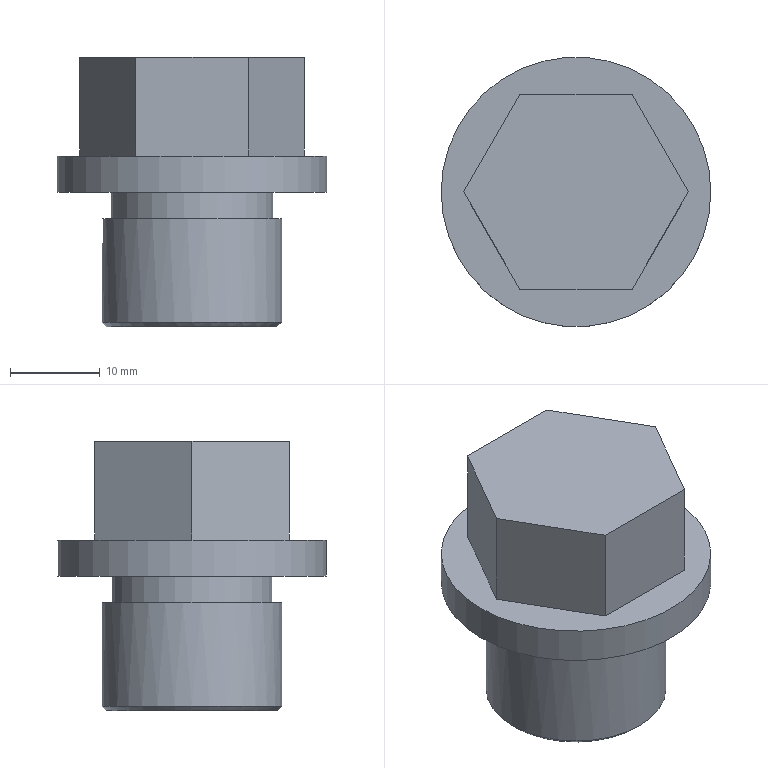Part | NX | features DATUM_CSYS 5, EXTRUDE 4, SKETCH 4, CHAMFER 1 | 1 solid | 15 faces | box 30 x 30 x 30 mm | volume 11818 mm3 | plane 11 | cylinder 3 | cone 1 | commonest cylinder face diameters 18 x1 20 x1 30 x1
STEP:
#1=CARTESIAN_POINT('',(-12.5,0.,0.));
#2=VERTEX_POINT('',#1);
#3=CARTESIAN_POINT('',(-6.25,-10.825,0.));
#4=VERTEX_POINT('',#3);
#5=CARTESIAN_POINT('',(-12.5,0.,0.));
#6=DIRECTION('',(0.5,-0.866,0.));
#7=VECTOR('',#6,1000.);
#8=LINE('',#5,#7);
#9=EDGE_CURVE('',#2,#4,#8,.T.);
#10=ORIENTED_EDGE('',*,*,#9,.T.);
#11=CARTESIAN_POINT('',(-6.25,-10.825,11.));
#12=VERTEX_POINT('',#11);
#13=CARTESIAN_POINT('',(-6.25,-10.825,11.));
#14=DIRECTION('',(0.,0.,-1.));
#15=VECTOR('',#14,1000.);
#16=LINE('',#13,#15);
#17=EDGE_CURVE('',#12,#4,#16,.T.);
#18=ORIENTED_EDGE('',*,*,#17,.F.);
#19=CARTESIAN_POINT('',(-12.5,0.,11.));
#20=VERTEX_POINT('',#19);
#21=CARTESIAN_POINT('',(-12.5,0.,11.));
#22=DIRECTION('',(0.5,-0.866,0.));
#23=VECTOR('',#22,1000.);
#24=LINE('',#21,#23);
#25=EDGE_CURVE('',#20,#12,#24,.T.);
#26=ORIENTED_EDGE('',*,*,#25,.F.);
#27=CARTESIAN_POINT('',(-12.5,0.,11.));
#28=DIRECTION('',(0.,0.,-1.));
#29=VECTOR('',#28,1000.);
#30=LINE('',#27,#29);
#31=EDGE_CURVE('',#20,#2,#30,.T.);
#32=ORIENTED_EDGE('',*,*,#31,.T.);
#33=EDGE_LOOP('',(#10,#18,#26,#32));
#34=FACE_BOUND('',#33,.T.);
#35=CARTESIAN_POINT('',(-12.5,0.,11.));
#36=DIRECTION('',(0.866,0.5,0.));
#37=DIRECTION('',(-0.5,0.866,0.));
#38=AXIS2_PLACEMENT_3D('',#35,#36,#37);
#39=PLANE('',#38);
#40=ADVANCED_FACE('',(#34),#39,.F.);
#41=CARTESIAN_POINT('',(6.25,-10.825,0.));
#42=VERTEX_POINT('',#41);
#43=CARTESIAN_POINT('',(-6.25,-10.825,0.));
#44=DIRECTION('',(1.,0.,0.));
#45=VECTOR('',#44,1000.);
#46=LINE('',#43,#45);
#47=EDGE_CURVE('',#4,#42,#46,.T.);
#48=ORIENTED_EDGE('',*,*,#47,.T.);
#49=CARTESIAN_POINT('',(6.25,-10.825,11.));
#50=VERTEX_POINT('',#49);
#51=CARTESIAN_POINT('',(6.25,-10.825,11.));
#52=DIRECTION('',(0.,0.,-1.));
#53=VECTOR('',#52,1000.);
#54=LINE('',#51,#53);
#55=EDGE_CURVE('',#50,#42,#54,.T.);
#56=ORIENTED_EDGE('',*,*,#55,.F.);
#57=CARTESIAN_POINT('',(-6.25,-10.825,11.));
#58=DIRECTION('',(1.,0.,0.));
#59=VECTOR('',#58,1000.);
#60=LINE('',#57,#59);
#61=EDGE_CURVE('',#12,#50,#60,.T.);
#62=ORIENTED_EDGE('',*,*,#61,.F.);
#63=ORIENTED_EDGE('',*,*,#17,.T.);
#64=EDGE_LOOP('',(#48,#56,#62,#63));
#65=FACE_BOUND('',#64,.T.);
#66=CARTESIAN_POINT('',(-6.25,-10.825,11.));
#67=DIRECTION('',(0.,1.,0.));
#68=DIRECTION('',(-1.,0.,0.));
#69=AXIS2_PLACEMENT_3D('',#66,#67,#68);
#70=PLANE('',#69);
#71=ADVANCED_FACE('',(#65),#70,.F.);
#72=CARTESIAN_POINT('',(12.5,0.,0.));
#73=VERTEX_POINT('',#72);
#74=CARTESIAN_POINT('',(6.25,-10.825,0.));
#75=DIRECTION('',(0.5,0.866,0.));
#76=VECTOR('',#75,1000.);
#77=LINE('',#74,#76);
#78=EDGE_CURVE('',#42,#73,#77,.T.);
#79=ORIENTED_EDGE('',*,*,#78,.T.);
#80=CARTESIAN_POINT('',(12.5,0.,11.));
#81=VERTEX_POINT('',#80);
#82=CARTESIAN_POINT('',(12.5,0.,11.));
#83=DIRECTION('',(0.,0.,-1.));
#84=VECTOR('',#83,1000.);
#85=LINE('',#82,#84);
#86=EDGE_CURVE('',#81,#73,#85,.T.);
#87=ORIENTED_EDGE('',*,*,#86,.F.);
#88=CARTESIAN_POINT('',(6.25,-10.825,11.));
#89=DIRECTION('',(0.5,0.866,0.));
#90=VECTOR('',#89,1000.);
#91=LINE('',#88,#90);
#92=EDGE_CURVE('',#50,#81,#91,.T.);
#93=ORIENTED_EDGE('',*,*,#92,.F.);
#94=ORIENTED_EDGE('',*,*,#55,.T.);
#95=EDGE_LOOP('',(#79,#87,#93,#94));
#96=FACE_BOUND('',#95,.T.);
#97=CARTESIAN_POINT('',(6.25,-10.825,11.));
#98=DIRECTION('',(-0.866,0.5,0.));
#99=DIRECTION('',(-0.5,-0.866,0.));
#100=AXIS2_PLACEMENT_3D('',#97,#98,#99);
#101=PLANE('',#100);
#102=ADVANCED_FACE('',(#96),#101,.F.);
#103=CARTESIAN_POINT('',(6.25,10.825,0.));
#104=VERTEX_POINT('',#103);
#105=CARTESIAN_POINT('',(12.5,0.,0.));
#106=DIRECTION('',(-0.5,0.866,0.));
#107=VECTOR('',#106,1000.);
#108=LINE('',#105,#107);
#109=EDGE_CURVE('',#73,#104,#108,.T.);
#110=ORIENTED_EDGE('',*,*,#109,.T.);
#111=CARTESIAN_POINT('',(6.25,10.825,11.));
#112=VERTEX_POINT('',#111);
#113=CARTESIAN_POINT('',(6.25,10.825,11.));
#114=DIRECTION('',(0.,0.,-1.));
#115=VECTOR('',#114,1000.);
#116=LINE('',#113,#115);
#117=EDGE_CURVE('',#112,#104,#116,.T.);
#118=ORIENTED_EDGE('',*,*,#117,.F.);
#119=CARTESIAN_POINT('',(12.5,0.,11.));
#120=DIRECTION('',(-0.5,0.866,0.));
#121=VECTOR('',#120,1000.);
#122=LINE('',#119,#121);
#123=EDGE_CURVE('',#81,#112,#122,.T.);
#124=ORIENTED_EDGE('',*,*,#123,.F.);
#125=ORIENTED_EDGE('',*,*,#86,.T.);
#126=EDGE_LOOP('',(#110,#118,#124,#125));
#127=FACE_BOUND('',#126,.T.);
#128=CARTESIAN_POINT('',(12.5,0.,11.));
#129=DIRECTION('',(-0.866,-0.5,0.));
#130=DIRECTION('',(0.5,-0.866,0.));
#131=AXIS2_PLACEMENT_3D('',#128,#129,#130);
#132=PLANE('',#131);
#133=ADVANCED_FACE('',(#127),#132,.F.);
#134=CARTESIAN_POINT('',(-6.25,10.825,0.));
#135=VERTEX_POINT('',#134);
#136=CARTESIAN_POINT('',(6.25,10.825,0.));
#137=DIRECTION('',(-1.,0.,0.));
#138=VECTOR('',#137,1000.);
#139=LINE('',#136,#138);
#140=EDGE_CURVE('',#104,#135,#139,.T.);
#141=ORIENTED_EDGE('',*,*,#140,.T.);
#142=CARTESIAN_POINT('',(-6.25,10.825,11.));
#143=VERTEX_POINT('',#142);
#144=CARTESIAN_POINT('',(-6.25,10.825,11.));
#145=DIRECTION('',(0.,0.,-1.));
#146=VECTOR('',#145,1000.);
#147=LINE('',#144,#146);
#148=EDGE_CURVE('',#143,#135,#147,.T.);
#149=ORIENTED_EDGE('',*,*,#148,.F.);
#150=CARTESIAN_POINT('',(6.25,10.825,11.));
#151=DIRECTION('',(-1.,0.,0.));
#152=VECTOR('',#151,1000.);
#153=LINE('',#150,#152);
#154=EDGE_CURVE('',#112,#143,#153,.T.);
#155=ORIENTED_EDGE('',*,*,#154,.F.);
#156=ORIENTED_EDGE('',*,*,#117,.T.);
#157=EDGE_LOOP('',(#141,#149,#155,#156));
#158=FACE_BOUND('',#157,.T.);
#159=CARTESIAN_POINT('',(6.25,10.825,11.));
#160=DIRECTION('',(0.,-1.,0.));
#161=DIRECTION('',(1.,0.,0.));
#162=AXIS2_PLACEMENT_3D('',#159,#160,#161);
#163=PLANE('',#162);
#164=ADVANCED_FACE('',(#158),#163,.F.);
#165=CARTESIAN_POINT('',(-6.25,10.825,0.));
#166=DIRECTION('',(-0.5,-0.866,0.));
#167=VECTOR('',#166,1000.);
#168=LINE('',#165,#167);
#169=EDGE_CURVE('',#135,#2,#168,.T.);
#170=ORIENTED_EDGE('',*,*,#169,.T.);
#171=ORIENTED_EDGE('',*,*,#31,.F.);
#172=CARTESIAN_POINT('',(-6.25,10.825,11.));
#173=DIRECTION('',(-0.5,-0.866,0.));
#174=VECTOR('',#173,1000.);
#175=LINE('',#172,#174);
#176=EDGE_CURVE('',#143,#20,#175,.T.);
#177=ORIENTED_EDGE('',*,*,#176,.F.);
#178=ORIENTED_EDGE('',*,*,#148,.T.);
#179=EDGE_LOOP('',(#170,#171,#177,#178));
#180=FACE_BOUND('',#179,.T.);
#181=CARTESIAN_POINT('',(-6.25,10.825,11.));
#182=DIRECTION('',(0.866,-0.5,0.));
#183=DIRECTION('',(0.5,0.866,0.));
#184=AXIS2_PLACEMENT_3D('',#181,#182,#183);
#185=PLANE('',#184);
#186=ADVANCED_FACE('',(#180),#185,.F.);
#187=ORIENTED_EDGE('',*,*,#25,.T.);
#188=ORIENTED_EDGE('',*,*,#61,.T.);
#189=ORIENTED_EDGE('',*,*,#92,.T.);
#190=ORIENTED_EDGE('',*,*,#123,.T.);
#191=ORIENTED_EDGE('',*,*,#154,.T.);
#192=ORIENTED_EDGE('',*,*,#176,.T.);
#193=EDGE_LOOP('',(#187,#188,#189,#190,#191,#192));
#194=FACE_BOUND('',#193,.T.);
#195=CARTESIAN_POINT('',(0.,0.,11.));
#196=DIRECTION('',(0.,0.,1.));
#197=DIRECTION('',(1.,0.,0.));
#198=AXIS2_PLACEMENT_3D('',#195,#196,#197);
#199=PLANE('',#198);
#200=ADVANCED_FACE('',(#194),#199,.T.);
#201=CARTESIAN_POINT('',(15.,0.,0.));
#202=VERTEX_POINT('',#201);
#203=CARTESIAN_POINT('',(0.,0.,0.));
#204=DIRECTION('',(0.,0.,1.));
#205=DIRECTION('',(1.,0.,0.));
#206=AXIS2_PLACEMENT_3D('',#203,#204,#205);
#207=CIRCLE('',#206,15.);
#208=EDGE_CURVE('',#202,#202,#207,.T.);
#209=ORIENTED_EDGE('',*,*,#208,.T.);
#210=EDGE_LOOP('',(#209));
#211=FACE_BOUND('',#210,.T.);
#212=ORIENTED_EDGE('',*,*,#9,.F.);
#213=ORIENTED_EDGE('',*,*,#169,.F.);
#214=ORIENTED_EDGE('',*,*,#140,.F.);
#215=ORIENTED_EDGE('',*,*,#109,.F.);
#216=ORIENTED_EDGE('',*,*,#78,.F.);
#217=ORIENTED_EDGE('',*,*,#47,.F.);
#218=EDGE_LOOP('',(#212,#213,#214,#215,#216,#217));
#219=FACE_BOUND('',#218,.T.);
#220=CARTESIAN_POINT('',(0.,0.,0.));
#221=DIRECTION('',(0.,0.,1.));
#222=DIRECTION('',(1.,0.,0.));
#223=AXIS2_PLACEMENT_3D('',#220,#221,#222);
#224=PLANE('',#223);
#225=ADVANCED_FACE('',(#211,#219),#224,.T.);
#226=CARTESIAN_POINT('',(15.,0.,-4.));
#227=VERTEX_POINT('',#226);
#228=CARTESIAN_POINT('',(0.,0.,-4.));
#229=DIRECTION('',(0.,0.,1.));
#230=DIRECTION('',(1.,0.,0.));
#231=AXIS2_PLACEMENT_3D('',#228,#229,#230);
#232=CIRCLE('',#231,15.);
#233=EDGE_CURVE('',#227,#227,#232,.T.);
#234=ORIENTED_EDGE('',*,*,#233,.T.);
#235=EDGE_LOOP('',(#234));
#236=FACE_BOUND('',#235,.T.);
#237=ORIENTED_EDGE('',*,*,#208,.F.);
#238=EDGE_LOOP('',(#237));
#239=FACE_BOUND('',#238,.T.);
#240=CARTESIAN_POINT('',(0.,0.,-4.));
#241=DIRECTION('',(0.,0.,1.));
#242=DIRECTION('',(1.,0.,0.));
#243=AXIS2_PLACEMENT_3D('',#240,#241,#242);
#244=CYLINDRICAL_SURFACE('',#243,15.);
#245=ADVANCED_FACE('',(#236,#239),#244,.T.);
#246=CARTESIAN_POINT('',(9.,0.,-4.));
#247=VERTEX_POINT('',#246);
#248=CARTESIAN_POINT('',(0.,0.,-4.));
#249=DIRECTION('',(0.,0.,-1.));
#250=DIRECTION('',(1.,0.,0.));
#251=AXIS2_PLACEMENT_3D('',#248,#249,#250);
#252=CIRCLE('',#251,9.);
#253=EDGE_CURVE('',#247,#247,#252,.T.);
#254=ORIENTED_EDGE('',*,*,#253,.F.);
#255=EDGE_LOOP('',(#254));
#256=FACE_BOUND('',#255,.T.);
#257=ORIENTED_EDGE('',*,*,#233,.F.);
#258=EDGE_LOOP('',(#257));
#259=FACE_BOUND('',#258,.T.);
#260=CARTESIAN_POINT('',(0.,0.,-4.));
#261=DIRECTION('',(0.,0.,1.));
#262=DIRECTION('',(1.,0.,0.));
#263=AXIS2_PLACEMENT_3D('',#260,#261,#262);
#264=PLANE('',#263);
#265=ADVANCED_FACE('',(#256,#259),#264,.F.);
#266=CARTESIAN_POINT('',(9.,0.,-7.));
#267=VERTEX_POINT('',#266);
#268=CARTESIAN_POINT('',(0.,0.,-7.));
#269=DIRECTION('',(0.,0.,-1.));
#270=DIRECTION('',(1.,0.,0.));
#271=AXIS2_PLACEMENT_3D('',#268,#269,#270);
#272=CIRCLE('',#271,9.);
#273=EDGE_CURVE('',#267,#267,#272,.T.);
#274=ORIENTED_EDGE('',*,*,#273,.F.);
#275=EDGE_LOOP('',(#274));
#276=FACE_BOUND('',#275,.T.);
#277=ORIENTED_EDGE('',*,*,#253,.T.);
#278=EDGE_LOOP('',(#277));
#279=FACE_BOUND('',#278,.T.);
#280=CARTESIAN_POINT('',(0.,0.,-7.));
#281=DIRECTION('',(0.,0.,1.));
#282=DIRECTION('',(1.,0.,0.));
#283=AXIS2_PLACEMENT_3D('',#280,#281,#282);
#284=CYLINDRICAL_SURFACE('',#283,9.);
#285=ADVANCED_FACE('',(#276,#279),#284,.T.);
#286=CARTESIAN_POINT('',(-10.,0.,-18.5));
#287=VERTEX_POINT('',#286);
#288=CARTESIAN_POINT('',(0.,0.,-18.5));
#289=DIRECTION('',(0.,0.,-1.));
#290=DIRECTION('',(-1.,0.,0.));
#291=AXIS2_PLACEMENT_3D('',#288,#289,#290);
#292=CIRCLE('',#291,10.);
#293=EDGE_CURVE('',#287,#287,#292,.F.);
#294=ORIENTED_EDGE('',*,*,#293,.T.);
#295=EDGE_LOOP('',(#294));
#296=FACE_BOUND('',#295,.T.);
#297=CARTESIAN_POINT('',(10.,0.,-7.));
#298=VERTEX_POINT('',#297);
#299=CARTESIAN_POINT('',(0.,0.,-7.));
#300=DIRECTION('',(0.,0.,-1.));
#301=DIRECTION('',(1.,0.,0.));
#302=AXIS2_PLACEMENT_3D('',#299,#300,#301);
#303=CIRCLE('',#302,10.);
#304=EDGE_CURVE('',#298,#298,#303,.T.);
#305=ORIENTED_EDGE('',*,*,#304,.T.);
#306=EDGE_LOOP('',(#305));
#307=FACE_BOUND('',#306,.T.);
#308=CARTESIAN_POINT('',(0.,0.,-19.));
#309=DIRECTION('',(0.,0.,1.));
#310=DIRECTION('',(1.,0.,0.));
#311=AXIS2_PLACEMENT_3D('',#308,#309,#310);
#312=CYLINDRICAL_SURFACE('',#311,10.);
#313=ADVANCED_FACE('',(#296,#307),#312,.T.);
#314=CARTESIAN_POINT('',(-9.5,0.,-19.));
#315=VERTEX_POINT('',#314);
#316=CARTESIAN_POINT('',(0.,0.,-19.));
#317=DIRECTION('',(0.,0.,-1.));
#318=DIRECTION('',(-1.,0.,0.));
#319=AXIS2_PLACEMENT_3D('',#316,#317,#318);
#320=CIRCLE('',#319,9.5);
#321=EDGE_CURVE('',#315,#315,#320,.T.);
#322=ORIENTED_EDGE('',*,*,#321,.T.);
#323=EDGE_LOOP('',(#322));
#324=FACE_BOUND('',#323,.T.);
#325=CARTESIAN_POINT('',(0.,0.,-19.));
#326=DIRECTION('',(0.,0.,-1.));
#327=DIRECTION('',(-1.,0.,0.));
#328=AXIS2_PLACEMENT_3D('',#325,#326,#327);
#329=PLANE('',#328);
#330=ADVANCED_FACE('',(#324),#329,.T.);
#331=ORIENTED_EDGE('',*,*,#273,.T.);
#332=EDGE_LOOP('',(#331));
#333=FACE_BOUND('',#332,.T.);
#334=ORIENTED_EDGE('',*,*,#304,.F.);
#335=EDGE_LOOP('',(#334));
#336=FACE_BOUND('',#335,.T.);
#337=CARTESIAN_POINT('',(0.,0.,-7.));
#338=DIRECTION('',(0.,0.,-1.));
#339=DIRECTION('',(-1.,0.,0.));
#340=AXIS2_PLACEMENT_3D('',#337,#338,#339);
#341=PLANE('',#340);
#342=ADVANCED_FACE('',(#333,#336),#341,.F.);
#343=ORIENTED_EDGE('',*,*,#293,.F.);
#344=EDGE_LOOP('',(#343));
#345=FACE_BOUND('',#344,.T.);
#346=ORIENTED_EDGE('',*,*,#321,.F.);
#347=EDGE_LOOP('',(#346));
#348=FACE_BOUND('',#347,.T.);
#349=CARTESIAN_POINT('',(0.,0.,-19.));
#350=DIRECTION('',(0.,0.,1.));
#351=DIRECTION('',(1.,0.,0.));
#352=AXIS2_PLACEMENT_3D('',#349,#350,#351);
#353=CONICAL_SURFACE('',#352,9.5,0.7854);
#354=ADVANCED_FACE('',(#345,#348),#353,.T.);
#355=CLOSED_SHELL('',(#40,#71,#102,#133,#164,#186,#200,#225,#245,#265,#285,#313,#330,#342,#354));
#356=MANIFOLD_SOLID_BREP('',#355);
#357=(LENGTH_UNIT()NAMED_UNIT(*)SI_UNIT(.MILLI.,.METRE.));
#358=UNCERTAINTY_MEASURE_WITH_UNIT(LENGTH_MEASURE(0.00001),#357,'','');
#359=(NAMED_UNIT(*)PLANE_ANGLE_UNIT()SI_UNIT($,.RADIAN.));
#360=(NAMED_UNIT(*)SI_UNIT($,.STERADIAN.)SOLID_ANGLE_UNIT());
#361=(GEOMETRIC_REPRESENTATION_CONTEXT(3)GLOBAL_UNCERTAINTY_ASSIGNED_CONTEXT((#358))GLOBAL_UNIT_ASSIGNED_CONTEXT((#357,#359,#360))REPRESENTATION_CONTEXT('',''));
#362=ADVANCED_BREP_SHAPE_REPRESENTATION('',(#356),#361);